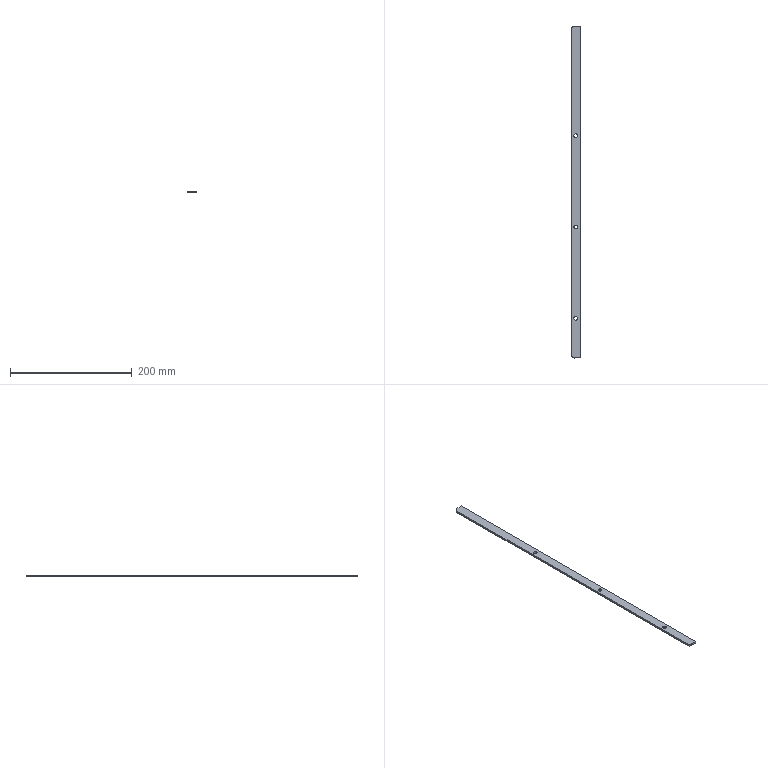Part | STEP file | Input 84 | 1 solid | 14 faces | box 15 x 545 x 3.2 mm | volume 25854 mm3 | cylinder 8 | plane 6 | commonest cylinder face diameters 6 x6 10 x2
STEP:
#1=CARTESIAN_POINT('',(0.,0.,0.));
#2=DIRECTION('',(0.,0.,1.));
#3=DIRECTION('',(1.,0.,0.));
#4=AXIS2_PLACEMENT_3D('',#1,#2,#3);
#5=CARTESIAN_POINT('',(4178.948,425.,2.794));
#6=VERTEX_POINT('',#5);
#7=CARTESIAN_POINT('',(4178.948,425.,-0.4063));
#8=VERTEX_POINT('',#7);
#9=CARTESIAN_POINT('',(4178.948,425.,2.795));
#10=DIRECTION('',(0.,0.,-1.));
#11=VECTOR('',#10,1.);
#12=LINE('',#9,#11);
#13=CARTESIAN_POINT('',(4175.948,425.,2.795));
#14=DIRECTION('',(0.,0.,-1.));
#15=DIRECTION('',(1.,0.,0.));
#16=AXIS2_PLACEMENT_3D('',#13,#14,#15);
#17=CYLINDRICAL_SURFACE('',#16,3.);
#18=CARTESIAN_POINT('',(6.283,0.));
#19=DIRECTION('',(0.,1.));
#20=VECTOR('',#19,1.);
#21=LINE('',#18,#20);
#22=(GEOMETRIC_REPRESENTATION_CONTEXT(2)PARAMETRIC_REPRESENTATION_CONTEXT()REPRESENTATION_CONTEXT('',''));
#23=DEFINITIONAL_REPRESENTATION('',(#21),#22);
#24=PCURVE('',#17,#23);
#25=CARTESIAN_POINT('',(4175.948,425.,2.795));
#26=DIRECTION('',(0.,0.,-1.));
#27=DIRECTION('',(1.,0.,0.));
#28=AXIS2_PLACEMENT_3D('',#25,#26,#27);
#29=CYLINDRICAL_SURFACE('',#28,3.);
#30=CARTESIAN_POINT('',(0.,0.));
#31=DIRECTION('',(0.,1.));
#32=VECTOR('',#31,1.);
#33=LINE('',#30,#32);
#34=(GEOMETRIC_REPRESENTATION_CONTEXT(2)PARAMETRIC_REPRESENTATION_CONTEXT()REPRESENTATION_CONTEXT('',''));
#35=DEFINITIONAL_REPRESENTATION('',(#33),#34);
#36=PCURVE('',#29,#35);
#37=SURFACE_CURVE('',#12,(#24,#36),.PCURVE_S1.);
#38=EDGE_CURVE('',#6,#8,#37,.T.);
#39=ORIENTED_EDGE('',*,*,#38,.T.);
#40=CARTESIAN_POINT('',(4172.948,425.,-0.4063));
#41=VERTEX_POINT('',#40);
#42=CARTESIAN_POINT('',(4175.948,425.,-0.4063));
#43=DIRECTION('',(0.,0.,1.));
#44=DIRECTION('',(1.,0.,0.));
#45=AXIS2_PLACEMENT_3D('',#42,#43,#44);
#46=CIRCLE('',#45,3.);
#47=CARTESIAN_POINT('',(6.283,3.201));
#48=DIRECTION('',(-1.,0.));
#49=VECTOR('',#48,1.);
#50=LINE('',#47,#49);
#51=(GEOMETRIC_REPRESENTATION_CONTEXT(2)PARAMETRIC_REPRESENTATION_CONTEXT()REPRESENTATION_CONTEXT('',''));
#52=DEFINITIONAL_REPRESENTATION('',(#50),#51);
#53=PCURVE('',#17,#52);
#54=CARTESIAN_POINT('',(4173.948,600.,-0.4063));
#55=DIRECTION('',(0.,0.,-1.));
#56=DIRECTION('',(1.,0.,0.));
#57=AXIS2_PLACEMENT_3D('',#54,#55,#56);
#58=PLANE('',#57);
#59=CARTESIAN_POINT('',(5.,175.));
#60=CARTESIAN_POINT('',(5.,169.804));
#61=CARTESIAN_POINT('',(0.5,172.402));
#62=CARTESIAN_POINT('',(-4.,175.));
#63=CARTESIAN_POINT('',(0.5,177.598));
#64=CARTESIAN_POINT('',(5.,180.196));
#65=CARTESIAN_POINT('',(5.,175.));
#66=(BOUNDED_CURVE()B_SPLINE_CURVE(2,(#59,#60,#61,#62,#63,#64,#65),.UNSPECIFIED.,.T.,.F.)B_SPLINE_CURVE_WITH_KNOTS((1,2,2,2,2,1),(-2.094,0.,2.094,4.189,6.283,8.378),.UNSPECIFIED.)CURVE()GEOMETRIC_REPRESENTATION_ITEM()RATIONAL_B_SPLINE_CURVE((1.,0.5,1.,0.5,1.,0.5,1.))REPRESENTATION_ITEM(''));
#67=(GEOMETRIC_REPRESENTATION_CONTEXT(2)PARAMETRIC_REPRESENTATION_CONTEXT()REPRESENTATION_CONTEXT('',''));
#68=DEFINITIONAL_REPRESENTATION('',(#66),#67);
#69=PCURVE('',#58,#68);
#70=SURFACE_CURVE('',#46,(#53,#69),.PCURVE_S1.);
#71=EDGE_CURVE('',#8,#41,#70,.T.);
#72=ORIENTED_EDGE('',*,*,#71,.T.);
#73=CARTESIAN_POINT('',(4172.948,425.,2.794));
#74=VERTEX_POINT('',#73);
#75=CARTESIAN_POINT('',(4172.948,425.,2.795));
#76=DIRECTION('',(0.,0.,-1.));
#77=VECTOR('',#76,1.);
#78=LINE('',#75,#77);
#79=CARTESIAN_POINT('',(3.142,0.));
#80=DIRECTION('',(0.,1.));
#81=VECTOR('',#80,1.);
#82=LINE('',#79,#81);
#83=(GEOMETRIC_REPRESENTATION_CONTEXT(2)PARAMETRIC_REPRESENTATION_CONTEXT()REPRESENTATION_CONTEXT('',''));
#84=DEFINITIONAL_REPRESENTATION('',(#82),#83);
#85=PCURVE('',#17,#84);
#86=CARTESIAN_POINT('',(3.142,0.));
#87=DIRECTION('',(0.,1.));
#88=VECTOR('',#87,1.);
#89=LINE('',#86,#88);
#90=(GEOMETRIC_REPRESENTATION_CONTEXT(2)PARAMETRIC_REPRESENTATION_CONTEXT()REPRESENTATION_CONTEXT('',''));
#91=DEFINITIONAL_REPRESENTATION('',(#89),#90);
#92=PCURVE('',#29,#91);
#93=SURFACE_CURVE('',#78,(#85,#92),.PCURVE_S1.);
#94=EDGE_CURVE('',#74,#41,#93,.T.);
#95=ORIENTED_EDGE('',*,*,#94,.F.);
#96=CARTESIAN_POINT('',(4175.948,425.,2.794));
#97=DIRECTION('',(0.,0.,-1.));
#98=DIRECTION('',(1.,0.,0.));
#99=AXIS2_PLACEMENT_3D('',#96,#97,#98);
#100=CIRCLE('',#99,3.);
#101=CARTESIAN_POINT('',(0.,0.001));
#102=DIRECTION('',(1.,0.));
#103=VECTOR('',#102,1.);
#104=LINE('',#101,#103);
#105=(GEOMETRIC_REPRESENTATION_CONTEXT(2)PARAMETRIC_REPRESENTATION_CONTEXT()REPRESENTATION_CONTEXT('',''));
#106=DEFINITIONAL_REPRESENTATION('',(#104),#105);
#107=PCURVE('',#17,#106);
#108=CARTESIAN_POINT('',(4173.948,600.,2.794));
#109=DIRECTION('',(0.,0.,-1.));
#110=DIRECTION('',(1.,0.,0.));
#111=AXIS2_PLACEMENT_3D('',#108,#109,#110);
#112=PLANE('',#111);
#113=CARTESIAN_POINT('',(2.,175.));
#114=DIRECTION('',(1.,0.));
#115=AXIS2_PLACEMENT_2D('',#113,#114);
#116=CIRCLE('',#115,3.);
#117=(GEOMETRIC_REPRESENTATION_CONTEXT(2)PARAMETRIC_REPRESENTATION_CONTEXT()REPRESENTATION_CONTEXT('',''));
#118=DEFINITIONAL_REPRESENTATION('',(#116),#117);
#119=PCURVE('',#112,#118);
#120=SURFACE_CURVE('',#100,(#107,#119),.PCURVE_S1.);
#121=EDGE_CURVE('',#74,#6,#120,.T.);
#122=ORIENTED_EDGE('',*,*,#121,.T.);
#123=EDGE_LOOP('',(#39,#72,#95,#122));
#124=FACE_BOUND('',#123,.F.);
#125=ADVANCED_FACE('',(#124),#17,.F.);
#126=CARTESIAN_POINT('',(4178.948,125.,2.794));
#127=VERTEX_POINT('',#126);
#128=CARTESIAN_POINT('',(4178.948,125.,-0.4063));
#129=VERTEX_POINT('',#128);
#130=CARTESIAN_POINT('',(4178.948,125.,2.795));
#131=DIRECTION('',(0.,0.,-1.));
#132=VECTOR('',#131,1.);
#133=LINE('',#130,#132);
#134=CARTESIAN_POINT('',(4175.948,125.,2.795));
#135=DIRECTION('',(0.,0.,-1.));
#136=DIRECTION('',(1.,0.,0.));
#137=AXIS2_PLACEMENT_3D('',#134,#135,#136);
#138=CYLINDRICAL_SURFACE('',#137,3.);
#139=CARTESIAN_POINT('',(6.283,0.));
#140=DIRECTION('',(0.,1.));
#141=VECTOR('',#140,1.);
#142=LINE('',#139,#141);
#143=(GEOMETRIC_REPRESENTATION_CONTEXT(2)PARAMETRIC_REPRESENTATION_CONTEXT()REPRESENTATION_CONTEXT('',''));
#144=DEFINITIONAL_REPRESENTATION('',(#142),#143);
#145=PCURVE('',#138,#144);
#146=CARTESIAN_POINT('',(4175.948,125.,2.795));
#147=DIRECTION('',(0.,0.,-1.));
#148=DIRECTION('',(1.,0.,0.));
#149=AXIS2_PLACEMENT_3D('',#146,#147,#148);
#150=CYLINDRICAL_SURFACE('',#149,3.);
#151=CARTESIAN_POINT('',(0.,0.));
#152=DIRECTION('',(0.,1.));
#153=VECTOR('',#152,1.);
#154=LINE('',#151,#153);
#155=(GEOMETRIC_REPRESENTATION_CONTEXT(2)PARAMETRIC_REPRESENTATION_CONTEXT()REPRESENTATION_CONTEXT('',''));
#156=DEFINITIONAL_REPRESENTATION('',(#154),#155);
#157=PCURVE('',#150,#156);
#158=SURFACE_CURVE('',#133,(#145,#157),.PCURVE_S1.);
#159=EDGE_CURVE('',#127,#129,#158,.T.);
#160=ORIENTED_EDGE('',*,*,#159,.T.);
#161=CARTESIAN_POINT('',(4172.948,125.,-0.4063));
#162=VERTEX_POINT('',#161);
#163=CARTESIAN_POINT('',(4175.948,125.,-0.4063));
#164=DIRECTION('',(0.,0.,1.));
#165=DIRECTION('',(1.,0.,0.));
#166=AXIS2_PLACEMENT_3D('',#163,#164,#165);
#167=CIRCLE('',#166,3.);
#168=CARTESIAN_POINT('',(6.283,3.201));
#169=DIRECTION('',(-1.,0.));
#170=VECTOR('',#169,1.);
#171=LINE('',#168,#170);
#172=(GEOMETRIC_REPRESENTATION_CONTEXT(2)PARAMETRIC_REPRESENTATION_CONTEXT()REPRESENTATION_CONTEXT('',''));
#173=DEFINITIONAL_REPRESENTATION('',(#171),#172);
#174=PCURVE('',#138,#173);
#175=CARTESIAN_POINT('',(5.,475.));
#176=CARTESIAN_POINT('',(5.,469.804));
#177=CARTESIAN_POINT('',(0.5,472.402));
#178=CARTESIAN_POINT('',(-4.,475.));
#179=CARTESIAN_POINT('',(0.5,477.598));
#180=CARTESIAN_POINT('',(5.,480.196));
#181=CARTESIAN_POINT('',(5.,475.));
#182=(BOUNDED_CURVE()B_SPLINE_CURVE(2,(#175,#176,#177,#178,#179,#180,#181),.UNSPECIFIED.,.T.,.F.)B_SPLINE_CURVE_WITH_KNOTS((1,2,2,2,2,1),(-2.094,0.,2.094,4.189,6.283,8.378),.UNSPECIFIED.)CURVE()GEOMETRIC_REPRESENTATION_ITEM()RATIONAL_B_SPLINE_CURVE((1.,0.5,1.,0.5,1.,0.5,1.))REPRESENTATION_ITEM(''));
#183=(GEOMETRIC_REPRESENTATION_CONTEXT(2)PARAMETRIC_REPRESENTATION_CONTEXT()REPRESENTATION_CONTEXT('',''));
#184=DEFINITIONAL_REPRESENTATION('',(#182),#183);
#185=PCURVE('',#58,#184);
#186=SURFACE_CURVE('',#167,(#174,#185),.PCURVE_S1.);
#187=EDGE_CURVE('',#129,#162,#186,.T.);
#188=ORIENTED_EDGE('',*,*,#187,.T.);
#189=CARTESIAN_POINT('',(4172.948,125.,2.794));
#190=VERTEX_POINT('',#189);
#191=CARTESIAN_POINT('',(4172.948,125.,2.795));
#192=DIRECTION('',(0.,0.,-1.));
#193=VECTOR('',#192,1.);
#194=LINE('',#191,#193);
#195=CARTESIAN_POINT('',(3.142,0.));
#196=DIRECTION('',(0.,1.));
#197=VECTOR('',#196,1.);
#198=LINE('',#195,#197);
#199=(GEOMETRIC_REPRESENTATION_CONTEXT(2)PARAMETRIC_REPRESENTATION_CONTEXT()REPRESENTATION_CONTEXT('',''));
#200=DEFINITIONAL_REPRESENTATION('',(#198),#199);
#201=PCURVE('',#138,#200);
#202=CARTESIAN_POINT('',(3.142,0.));
#203=DIRECTION('',(0.,1.));
#204=VECTOR('',#203,1.);
#205=LINE('',#202,#204);
#206=(GEOMETRIC_REPRESENTATION_CONTEXT(2)PARAMETRIC_REPRESENTATION_CONTEXT()REPRESENTATION_CONTEXT('',''));
#207=DEFINITIONAL_REPRESENTATION('',(#205),#206);
#208=PCURVE('',#150,#207);
#209=SURFACE_CURVE('',#194,(#201,#208),.PCURVE_S1.);
#210=EDGE_CURVE('',#190,#162,#209,.T.);
#211=ORIENTED_EDGE('',*,*,#210,.F.);
#212=CARTESIAN_POINT('',(4175.948,125.,2.794));
#213=DIRECTION('',(0.,0.,-1.));
#214=DIRECTION('',(1.,0.,0.));
#215=AXIS2_PLACEMENT_3D('',#212,#213,#214);
#216=CIRCLE('',#215,3.);
#217=CARTESIAN_POINT('',(0.,0.001));
#218=DIRECTION('',(1.,0.));
#219=VECTOR('',#218,1.);
#220=LINE('',#217,#219);
#221=(GEOMETRIC_REPRESENTATION_CONTEXT(2)PARAMETRIC_REPRESENTATION_CONTEXT()REPRESENTATION_CONTEXT('',''));
#222=DEFINITIONAL_REPRESENTATION('',(#220),#221);
#223=PCURVE('',#138,#222);
#224=CARTESIAN_POINT('',(2.,475.));
#225=DIRECTION('',(1.,0.));
#226=AXIS2_PLACEMENT_2D('',#224,#225);
#227=CIRCLE('',#226,3.);
#228=(GEOMETRIC_REPRESENTATION_CONTEXT(2)PARAMETRIC_REPRESENTATION_CONTEXT()REPRESENTATION_CONTEXT('',''));
#229=DEFINITIONAL_REPRESENTATION('',(#227),#228);
#230=PCURVE('',#112,#229);
#231=SURFACE_CURVE('',#216,(#223,#230),.PCURVE_S1.);
#232=EDGE_CURVE('',#190,#127,#231,.T.);
#233=ORIENTED_EDGE('',*,*,#232,.T.);
#234=EDGE_LOOP('',(#160,#188,#211,#233));
#235=FACE_BOUND('',#234,.F.);
#236=ADVANCED_FACE('',(#235),#138,.F.);
#237=CARTESIAN_POINT('',(4178.948,275.,2.794));
#238=VERTEX_POINT('',#237);
#239=CARTESIAN_POINT('',(4178.948,275.,-0.4063));
#240=VERTEX_POINT('',#239);
#241=CARTESIAN_POINT('',(4178.948,275.,2.795));
#242=DIRECTION('',(0.,0.,-1.));
#243=VECTOR('',#242,1.);
#244=LINE('',#241,#243);
#245=CARTESIAN_POINT('',(4175.948,275.,2.795));
#246=DIRECTION('',(0.,0.,-1.));
#247=DIRECTION('',(1.,0.,0.));
#248=AXIS2_PLACEMENT_3D('',#245,#246,#247);
#249=CYLINDRICAL_SURFACE('',#248,3.);
#250=CARTESIAN_POINT('',(6.283,0.));
#251=DIRECTION('',(0.,1.));
#252=VECTOR('',#251,1.);
#253=LINE('',#250,#252);
#254=(GEOMETRIC_REPRESENTATION_CONTEXT(2)PARAMETRIC_REPRESENTATION_CONTEXT()REPRESENTATION_CONTEXT('',''));
#255=DEFINITIONAL_REPRESENTATION('',(#253),#254);
#256=PCURVE('',#249,#255);
#257=CARTESIAN_POINT('',(4175.948,275.,2.795));
#258=DIRECTION('',(0.,0.,-1.));
#259=DIRECTION('',(1.,0.,0.));
#260=AXIS2_PLACEMENT_3D('',#257,#258,#259);
#261=CYLINDRICAL_SURFACE('',#260,3.);
#262=CARTESIAN_POINT('',(0.,0.));
#263=DIRECTION('',(0.,1.));
#264=VECTOR('',#263,1.);
#265=LINE('',#262,#264);
#266=(GEOMETRIC_REPRESENTATION_CONTEXT(2)PARAMETRIC_REPRESENTATION_CONTEXT()REPRESENTATION_CONTEXT('',''));
#267=DEFINITIONAL_REPRESENTATION('',(#265),#266);
#268=PCURVE('',#261,#267);
#269=SURFACE_CURVE('',#244,(#256,#268),.PCURVE_S1.);
#270=EDGE_CURVE('',#238,#240,#269,.T.);
#271=ORIENTED_EDGE('',*,*,#270,.T.);
#272=CARTESIAN_POINT('',(4172.948,275.,-0.4063));
#273=VERTEX_POINT('',#272);
#274=CARTESIAN_POINT('',(4175.948,275.,-0.4063));
#275=DIRECTION('',(0.,0.,1.));
#276=DIRECTION('',(1.,0.,0.));
#277=AXIS2_PLACEMENT_3D('',#274,#275,#276);
#278=CIRCLE('',#277,3.);
#279=CARTESIAN_POINT('',(6.283,3.201));
#280=DIRECTION('',(-1.,0.));
#281=VECTOR('',#280,1.);
#282=LINE('',#279,#281);
#283=(GEOMETRIC_REPRESENTATION_CONTEXT(2)PARAMETRIC_REPRESENTATION_CONTEXT()REPRESENTATION_CONTEXT('',''));
#284=DEFINITIONAL_REPRESENTATION('',(#282),#283);
#285=PCURVE('',#249,#284);
#286=CARTESIAN_POINT('',(5.,325.));
#287=CARTESIAN_POINT('',(5.,319.804));
#288=CARTESIAN_POINT('',(0.5,322.402));
#289=CARTESIAN_POINT('',(-4.,325.));
#290=CARTESIAN_POINT('',(0.5,327.598));
#291=CARTESIAN_POINT('',(5.,330.196));
#292=CARTESIAN_POINT('',(5.,325.));
#293=(BOUNDED_CURVE()B_SPLINE_CURVE(2,(#286,#287,#288,#289,#290,#291,#292),.UNSPECIFIED.,.T.,.F.)B_SPLINE_CURVE_WITH_KNOTS((1,2,2,2,2,1),(-2.094,0.,2.094,4.189,6.283,8.378),.UNSPECIFIED.)CURVE()GEOMETRIC_REPRESENTATION_ITEM()RATIONAL_B_SPLINE_CURVE((1.,0.5,1.,0.5,1.,0.5,1.))REPRESENTATION_ITEM(''));
#294=(GEOMETRIC_REPRESENTATION_CONTEXT(2)PARAMETRIC_REPRESENTATION_CONTEXT()REPRESENTATION_CONTEXT('',''));
#295=DEFINITIONAL_REPRESENTATION('',(#293),#294);
#296=PCURVE('',#58,#295);
#297=SURFACE_CURVE('',#278,(#285,#296),.PCURVE_S1.);
#298=EDGE_CURVE('',#240,#273,#297,.T.);
#299=ORIENTED_EDGE('',*,*,#298,.T.);
#300=CARTESIAN_POINT('',(4172.948,275.,2.794));
#301=VERTEX_POINT('',#300);
#302=CARTESIAN_POINT('',(4172.948,275.,2.795));
#303=DIRECTION('',(0.,0.,-1.));
#304=VECTOR('',#303,1.);
#305=LINE('',#302,#304);
#306=CARTESIAN_POINT('',(3.142,0.));
#307=DIRECTION('',(0.,1.));
#308=VECTOR('',#307,1.);
#309=LINE('',#306,#308);
#310=(GEOMETRIC_REPRESENTATION_CONTEXT(2)PARAMETRIC_REPRESENTATION_CONTEXT()REPRESENTATION_CONTEXT('',''));
#311=DEFINITIONAL_REPRESENTATION('',(#309),#310);
#312=PCURVE('',#249,#311);
#313=CARTESIAN_POINT('',(3.142,0.));
#314=DIRECTION('',(0.,1.));
#315=VECTOR('',#314,1.);
#316=LINE('',#313,#315);
#317=(GEOMETRIC_REPRESENTATION_CONTEXT(2)PARAMETRIC_REPRESENTATION_CONTEXT()REPRESENTATION_CONTEXT('',''));
#318=DEFINITIONAL_REPRESENTATION('',(#316),#317);
#319=PCURVE('',#261,#318);
#320=SURFACE_CURVE('',#305,(#312,#319),.PCURVE_S1.);
#321=EDGE_CURVE('',#301,#273,#320,.T.);
#322=ORIENTED_EDGE('',*,*,#321,.F.);
#323=CARTESIAN_POINT('',(4175.948,275.,2.794));
#324=DIRECTION('',(0.,0.,-1.));
#325=DIRECTION('',(1.,0.,0.));
#326=AXIS2_PLACEMENT_3D('',#323,#324,#325);
#327=CIRCLE('',#326,3.);
#328=CARTESIAN_POINT('',(0.,0.001));
#329=DIRECTION('',(1.,0.));
#330=VECTOR('',#329,1.);
#331=LINE('',#328,#330);
#332=(GEOMETRIC_REPRESENTATION_CONTEXT(2)PARAMETRIC_REPRESENTATION_CONTEXT()REPRESENTATION_CONTEXT('',''));
#333=DEFINITIONAL_REPRESENTATION('',(#331),#332);
#334=PCURVE('',#249,#333);
#335=CARTESIAN_POINT('',(2.,325.));
#336=DIRECTION('',(1.,0.));
#337=AXIS2_PLACEMENT_2D('',#335,#336);
#338=CIRCLE('',#337,3.);
#339=(GEOMETRIC_REPRESENTATION_CONTEXT(2)PARAMETRIC_REPRESENTATION_CONTEXT()REPRESENTATION_CONTEXT('',''));
#340=DEFINITIONAL_REPRESENTATION('',(#338),#339);
#341=PCURVE('',#112,#340);
#342=SURFACE_CURVE('',#327,(#334,#341),.PCURVE_S1.);
#343=EDGE_CURVE('',#301,#238,#342,.T.);
#344=ORIENTED_EDGE('',*,*,#343,.T.);
#345=EDGE_LOOP('',(#271,#299,#322,#344));
#346=FACE_BOUND('',#345,.F.);
#347=ADVANCED_FACE('',(#346),#249,.F.);
#348=CARTESIAN_POINT('',(4183.948,605.,-0.4063));
#349=VERTEX_POINT('',#348);
#350=CARTESIAN_POINT('',(4173.948,605.,-0.4063));
#351=VERTEX_POINT('',#350);
#352=CARTESIAN_POINT('',(4183.948,605.,-0.4063));
#353=DIRECTION('',(-1.,0.,0.));
#354=VECTOR('',#353,1.);
#355=LINE('',#352,#354);
#356=CARTESIAN_POINT('',(4183.948,605.,2.794));
#357=DIRECTION('',(0.,1.,0.));
#358=DIRECTION('',(-1.,0.,0.));
#359=AXIS2_PLACEMENT_3D('',#356,#357,#358);
#360=PLANE('',#359);
#361=CARTESIAN_POINT('',(0.,-3.2));
#362=DIRECTION('',(1.,0.));
#363=VECTOR('',#362,1.);
#364=LINE('',#361,#363);
#365=(GEOMETRIC_REPRESENTATION_CONTEXT(2)PARAMETRIC_REPRESENTATION_CONTEXT()REPRESENTATION_CONTEXT('',''));
#366=DEFINITIONAL_REPRESENTATION('',(#364),#365);
#367=PCURVE('',#360,#366);
#368=CARTESIAN_POINT('',(10.,-5.));
#369=DIRECTION('',(-1.,0.));
#370=VECTOR('',#369,1.);
#371=LINE('',#368,#370);
#372=(GEOMETRIC_REPRESENTATION_CONTEXT(2)PARAMETRIC_REPRESENTATION_CONTEXT()REPRESENTATION_CONTEXT('',''));
#373=DEFINITIONAL_REPRESENTATION('',(#371),#372);
#374=PCURVE('',#58,#373);
#375=SURFACE_CURVE('',#355,(#367,#374),.PCURVE_S1.);
#376=EDGE_CURVE('',#349,#351,#375,.T.);
#377=ORIENTED_EDGE('',*,*,#376,.T.);
#378=CARTESIAN_POINT('',(4173.948,605.,2.794));
#379=VERTEX_POINT('',#378);
#380=CARTESIAN_POINT('',(4173.948,605.,2.794));
#381=DIRECTION('',(0.,0.,-1.));
#382=VECTOR('',#381,1.);
#383=LINE('',#380,#382);
#384=CARTESIAN_POINT('',(10.,0.));
#385=DIRECTION('',(0.,-1.));
#386=VECTOR('',#385,1.);
#387=LINE('',#384,#386);
#388=(GEOMETRIC_REPRESENTATION_CONTEXT(2)PARAMETRIC_REPRESENTATION_CONTEXT()REPRESENTATION_CONTEXT('',''));
#389=DEFINITIONAL_REPRESENTATION('',(#387),#388);
#390=PCURVE('',#360,#389);
#391=CARTESIAN_POINT('',(4173.948,600.,2.794));
#392=DIRECTION('',(0.,0.,-1.));
#393=DIRECTION('',(1.,0.,0.));
#394=AXIS2_PLACEMENT_3D('',#391,#392,#393);
#395=CYLINDRICAL_SURFACE('',#394,5.);
#396=CARTESIAN_POINT('',(4.712,0.));
#397=DIRECTION('',(0.,1.));
#398=VECTOR('',#397,1.);
#399=LINE('',#396,#398);
#400=(GEOMETRIC_REPRESENTATION_CONTEXT(2)PARAMETRIC_REPRESENTATION_CONTEXT()REPRESENTATION_CONTEXT('',''));
#401=DEFINITIONAL_REPRESENTATION('',(#399),#400);
#402=PCURVE('',#395,#401);
#403=SURFACE_CURVE('',#383,(#390,#402),.PCURVE_S1.);
#404=EDGE_CURVE('',#379,#351,#403,.T.);
#405=ORIENTED_EDGE('',*,*,#404,.F.);
#406=CARTESIAN_POINT('',(4183.948,605.,2.794));
#407=VERTEX_POINT('',#406);
#408=CARTESIAN_POINT('',(4183.948,605.,2.794));
#409=DIRECTION('',(-1.,0.,0.));
#410=VECTOR('',#409,1.);
#411=LINE('',#408,#410);
#412=CARTESIAN_POINT('',(0.,0.));
#413=DIRECTION('',(1.,0.));
#414=VECTOR('',#413,1.);
#415=LINE('',#412,#414);
#416=(GEOMETRIC_REPRESENTATION_CONTEXT(2)PARAMETRIC_REPRESENTATION_CONTEXT()REPRESENTATION_CONTEXT('',''));
#417=DEFINITIONAL_REPRESENTATION('',(#415),#416);
#418=PCURVE('',#360,#417);
#419=CARTESIAN_POINT('',(10.,-5.));
#420=DIRECTION('',(-1.,0.));
#421=VECTOR('',#420,1.);
#422=LINE('',#419,#421);
#423=(GEOMETRIC_REPRESENTATION_CONTEXT(2)PARAMETRIC_REPRESENTATION_CONTEXT()REPRESENTATION_CONTEXT('',''));
#424=DEFINITIONAL_REPRESENTATION('',(#422),#423);
#425=PCURVE('',#112,#424);
#426=SURFACE_CURVE('',#411,(#418,#425),.PCURVE_S1.);
#427=EDGE_CURVE('',#407,#379,#426,.T.);
#428=ORIENTED_EDGE('',*,*,#427,.F.);
#429=CARTESIAN_POINT('',(4183.948,605.,2.794));
#430=DIRECTION('',(0.,0.,-1.));
#431=VECTOR('',#430,1.);
#432=LINE('',#429,#431);
#433=CARTESIAN_POINT('',(0.,0.));
#434=DIRECTION('',(0.,-1.));
#435=VECTOR('',#434,1.);
#436=LINE('',#433,#435);
#437=(GEOMETRIC_REPRESENTATION_CONTEXT(2)PARAMETRIC_REPRESENTATION_CONTEXT()REPRESENTATION_CONTEXT('',''));
#438=DEFINITIONAL_REPRESENTATION('',(#436),#437);
#439=PCURVE('',#360,#438);
#440=CARTESIAN_POINT('',(4183.948,605.,2.794));
#441=DIRECTION('',(1.,0.,0.));
#442=DIRECTION('',(0.,1.,0.));
#443=AXIS2_PLACEMENT_3D('',#440,#441,#442);
#444=PLANE('',#443);
#445=CARTESIAN_POINT('',(0.,0.));
#446=DIRECTION('',(0.,-1.));
#447=VECTOR('',#446,1.);
#448=LINE('',#445,#447);
#449=(GEOMETRIC_REPRESENTATION_CONTEXT(2)PARAMETRIC_REPRESENTATION_CONTEXT()REPRESENTATION_CONTEXT('',''));
#450=DEFINITIONAL_REPRESENTATION('',(#448),#449);
#451=PCURVE('',#444,#450);
#452=SURFACE_CURVE('',#432,(#439,#451),.PCURVE_S1.);
#453=EDGE_CURVE('',#407,#349,#452,.T.);
#454=ORIENTED_EDGE('',*,*,#453,.T.);
#455=EDGE_LOOP('',(#377,#405,#428,#454));
#456=FACE_BOUND('',#455,.T.);
#457=ADVANCED_FACE('',(#456),#360,.T.);
#458=CARTESIAN_POINT('',(4183.948,60.,-0.4063));
#459=VERTEX_POINT('',#458);
#460=CARTESIAN_POINT('',(4183.948,605.,-0.4063));
#461=DIRECTION('',(0.,1.,0.));
#462=VECTOR('',#461,1.);
#463=LINE('',#460,#462);
#464=CARTESIAN_POINT('',(0.,-3.2));
#465=DIRECTION('',(1.,0.));
#466=VECTOR('',#465,1.);
#467=LINE('',#464,#466);
#468=(GEOMETRIC_REPRESENTATION_CONTEXT(2)PARAMETRIC_REPRESENTATION_CONTEXT()REPRESENTATION_CONTEXT('',''));
#469=DEFINITIONAL_REPRESENTATION('',(#467),#468);
#470=PCURVE('',#444,#469);
#471=CARTESIAN_POINT('',(10.,-5.));
#472=DIRECTION('',(0.,-1.));
#473=VECTOR('',#472,1.);
#474=LINE('',#471,#473);
#475=(GEOMETRIC_REPRESENTATION_CONTEXT(2)PARAMETRIC_REPRESENTATION_CONTEXT()REPRESENTATION_CONTEXT('',''));
#476=DEFINITIONAL_REPRESENTATION('',(#474),#475);
#477=PCURVE('',#58,#476);
#478=SURFACE_CURVE('',#463,(#470,#477),.PCURVE_S1.);
#479=EDGE_CURVE('',#459,#349,#478,.T.);
#480=ORIENTED_EDGE('',*,*,#479,.T.);
#481=ORIENTED_EDGE('',*,*,#453,.F.);
#482=CARTESIAN_POINT('',(4183.948,60.,2.794));
#483=VERTEX_POINT('',#482);
#484=CARTESIAN_POINT('',(4183.948,605.,2.794));
#485=DIRECTION('',(0.,1.,0.));
#486=VECTOR('',#485,1.);
#487=LINE('',#484,#486);
#488=CARTESIAN_POINT('',(0.,0.));
#489=DIRECTION('',(1.,0.));
#490=VECTOR('',#489,1.);
#491=LINE('',#488,#490);
#492=(GEOMETRIC_REPRESENTATION_CONTEXT(2)PARAMETRIC_REPRESENTATION_CONTEXT()REPRESENTATION_CONTEXT('',''));
#493=DEFINITIONAL_REPRESENTATION('',(#491),#492);
#494=PCURVE('',#444,#493);
#495=CARTESIAN_POINT('',(10.,-5.));
#496=DIRECTION('',(0.,-1.));
#497=VECTOR('',#496,1.);
#498=LINE('',#495,#497);
#499=(GEOMETRIC_REPRESENTATION_CONTEXT(2)PARAMETRIC_REPRESENTATION_CONTEXT()REPRESENTATION_CONTEXT('',''));
#500=DEFINITIONAL_REPRESENTATION('',(#498),#499);
#501=PCURVE('',#112,#500);
#502=SURFACE_CURVE('',#487,(#494,#501),.PCURVE_S1.);
#503=EDGE_CURVE('',#483,#407,#502,.T.);
#504=ORIENTED_EDGE('',*,*,#503,.F.);
#505=CARTESIAN_POINT('',(4183.948,60.,2.794));
#506=DIRECTION('',(0.,0.,-1.));
#507=VECTOR('',#506,1.);
#508=LINE('',#505,#507);
#509=CARTESIAN_POINT('',(-545.,0.));
#510=DIRECTION('',(0.,-1.));
#511=VECTOR('',#510,1.);
#512=LINE('',#509,#511);
#513=(GEOMETRIC_REPRESENTATION_CONTEXT(2)PARAMETRIC_REPRESENTATION_CONTEXT()REPRESENTATION_CONTEXT('',''));
#514=DEFINITIONAL_REPRESENTATION('',(#512),#513);
#515=PCURVE('',#444,#514);
#516=CARTESIAN_POINT('',(4183.948,60.,2.794));
#517=DIRECTION('',(0.,-1.,0.));
#518=DIRECTION('',(1.,0.,0.));
#519=AXIS2_PLACEMENT_3D('',#516,#517,#518);
#520=PLANE('',#519);
#521=CARTESIAN_POINT('',(0.,0.));
#522=DIRECTION('',(0.,-1.));
#523=VECTOR('',#522,1.);
#524=LINE('',#521,#523);
#525=(GEOMETRIC_REPRESENTATION_CONTEXT(2)PARAMETRIC_REPRESENTATION_CONTEXT()REPRESENTATION_CONTEXT('',''));
#526=DEFINITIONAL_REPRESENTATION('',(#524),#525);
#527=PCURVE('',#520,#526);
#528=SURFACE_CURVE('',#508,(#515,#527),.PCURVE_S1.);
#529=EDGE_CURVE('',#483,#459,#528,.T.);
#530=ORIENTED_EDGE('',*,*,#529,.T.);
#531=EDGE_LOOP('',(#480,#481,#504,#530));
#532=FACE_BOUND('',#531,.T.);
#533=ADVANCED_FACE('',(#532),#444,.T.);
#534=CARTESIAN_POINT('',(4173.948,60.,-0.4063));
#535=VERTEX_POINT('',#534);
#536=CARTESIAN_POINT('',(4183.948,60.,-0.4063));
#537=DIRECTION('',(1.,0.,0.));
#538=VECTOR('',#537,1.);
#539=LINE('',#536,#538);
#540=CARTESIAN_POINT('',(0.,-3.2));
#541=DIRECTION('',(1.,0.));
#542=VECTOR('',#541,1.);
#543=LINE('',#540,#542);
#544=(GEOMETRIC_REPRESENTATION_CONTEXT(2)PARAMETRIC_REPRESENTATION_CONTEXT()REPRESENTATION_CONTEXT('',''));
#545=DEFINITIONAL_REPRESENTATION('',(#543),#544);
#546=PCURVE('',#520,#545);
#547=CARTESIAN_POINT('',(10.,540.));
#548=DIRECTION('',(1.,0.));
#549=VECTOR('',#548,1.);
#550=LINE('',#547,#549);
#551=(GEOMETRIC_REPRESENTATION_CONTEXT(2)PARAMETRIC_REPRESENTATION_CONTEXT()REPRESENTATION_CONTEXT('',''));
#552=DEFINITIONAL_REPRESENTATION('',(#550),#551);
#553=PCURVE('',#58,#552);
#554=SURFACE_CURVE('',#539,(#546,#553),.PCURVE_S1.);
#555=EDGE_CURVE('',#535,#459,#554,.T.);
#556=ORIENTED_EDGE('',*,*,#555,.T.);
#557=ORIENTED_EDGE('',*,*,#529,.F.);
#558=CARTESIAN_POINT('',(4173.948,60.,2.794));
#559=VERTEX_POINT('',#558);
#560=CARTESIAN_POINT('',(4183.948,60.,2.794));
#561=DIRECTION('',(1.,0.,0.));
#562=VECTOR('',#561,1.);
#563=LINE('',#560,#562);
#564=CARTESIAN_POINT('',(0.,0.));
#565=DIRECTION('',(1.,0.));
#566=VECTOR('',#565,1.);
#567=LINE('',#564,#566);
#568=(GEOMETRIC_REPRESENTATION_CONTEXT(2)PARAMETRIC_REPRESENTATION_CONTEXT()REPRESENTATION_CONTEXT('',''));
#569=DEFINITIONAL_REPRESENTATION('',(#567),#568);
#570=PCURVE('',#520,#569);
#571=CARTESIAN_POINT('',(10.,540.));
#572=DIRECTION('',(1.,0.));
#573=VECTOR('',#572,1.);
#574=LINE('',#571,#573);
#575=(GEOMETRIC_REPRESENTATION_CONTEXT(2)PARAMETRIC_REPRESENTATION_CONTEXT()REPRESENTATION_CONTEXT('',''));
#576=DEFINITIONAL_REPRESENTATION('',(#574),#575);
#577=PCURVE('',#112,#576);
#578=SURFACE_CURVE('',#563,(#570,#577),.PCURVE_S1.);
#579=EDGE_CURVE('',#559,#483,#578,.T.);
#580=ORIENTED_EDGE('',*,*,#579,.F.);
#581=CARTESIAN_POINT('',(4173.948,60.,2.794));
#582=DIRECTION('',(0.,0.,-1.));
#583=VECTOR('',#582,1.);
#584=LINE('',#581,#583);
#585=CARTESIAN_POINT('',(-10.,0.));
#586=DIRECTION('',(0.,-1.));
#587=VECTOR('',#586,1.);
#588=LINE('',#585,#587);
#589=(GEOMETRIC_REPRESENTATION_CONTEXT(2)PARAMETRIC_REPRESENTATION_CONTEXT()REPRESENTATION_CONTEXT('',''));
#590=DEFINITIONAL_REPRESENTATION('',(#588),#589);
#591=PCURVE('',#520,#590);
#592=CARTESIAN_POINT('',(4173.948,65.,2.794));
#593=DIRECTION('',(0.,0.,-1.));
#594=DIRECTION('',(1.,0.,0.));
#595=AXIS2_PLACEMENT_3D('',#592,#593,#594);
#596=CYLINDRICAL_SURFACE('',#595,5.);
#597=CARTESIAN_POINT('',(1.571,0.));
#598=DIRECTION('',(0.,1.));
#599=VECTOR('',#598,1.);
#600=LINE('',#597,#599);
#601=(GEOMETRIC_REPRESENTATION_CONTEXT(2)PARAMETRIC_REPRESENTATION_CONTEXT()REPRESENTATION_CONTEXT('',''));
#602=DEFINITIONAL_REPRESENTATION('',(#600),#601);
#603=PCURVE('',#596,#602);
#604=SURFACE_CURVE('',#584,(#591,#603),.PCURVE_S1.);
#605=EDGE_CURVE('',#559,#535,#604,.T.);
#606=ORIENTED_EDGE('',*,*,#605,.T.);
#607=EDGE_LOOP('',(#556,#557,#580,#606));
#608=FACE_BOUND('',#607,.T.);
#609=ADVANCED_FACE('',(#608),#520,.T.);
#610=CARTESIAN_POINT('',(4168.948,65.,-0.4063));
#611=VERTEX_POINT('',#610);
#612=CARTESIAN_POINT('',(4173.948,65.,-0.4063));
#613=DIRECTION('',(0.,0.,1.));
#614=DIRECTION('',(1.,0.,0.));
#615=AXIS2_PLACEMENT_3D('',#612,#613,#614);
#616=CIRCLE('',#615,5.);
#617=CARTESIAN_POINT('',(6.283,3.2));
#618=DIRECTION('',(-1.,0.));
#619=VECTOR('',#618,1.);
#620=LINE('',#617,#619);
#621=(GEOMETRIC_REPRESENTATION_CONTEXT(2)PARAMETRIC_REPRESENTATION_CONTEXT()REPRESENTATION_CONTEXT('',''));
#622=DEFINITIONAL_REPRESENTATION('',(#620),#621);
#623=PCURVE('',#596,#622);
#624=CARTESIAN_POINT('',(5.,535.));
#625=CARTESIAN_POINT('',(5.,526.34));
#626=CARTESIAN_POINT('',(-2.5,530.67));
#627=CARTESIAN_POINT('',(-10.,535.));
#628=CARTESIAN_POINT('',(-2.5,539.33));
#629=CARTESIAN_POINT('',(5.,543.66));
#630=CARTESIAN_POINT('',(5.,535.));
#631=(BOUNDED_CURVE()B_SPLINE_CURVE(2,(#624,#625,#626,#627,#628,#629,#630),.UNSPECIFIED.,.T.,.F.)B_SPLINE_CURVE_WITH_KNOTS((1,2,2,2,2,1),(-2.094,0.,2.094,4.189,6.283,8.378),.UNSPECIFIED.)CURVE()GEOMETRIC_REPRESENTATION_ITEM()RATIONAL_B_SPLINE_CURVE((1.,0.5,1.,0.5,1.,0.5,1.))REPRESENTATION_ITEM(''));
#632=(GEOMETRIC_REPRESENTATION_CONTEXT(2)PARAMETRIC_REPRESENTATION_CONTEXT()REPRESENTATION_CONTEXT('',''));
#633=DEFINITIONAL_REPRESENTATION('',(#631),#632);
#634=PCURVE('',#58,#633);
#635=SURFACE_CURVE('',#616,(#623,#634),.PCURVE_S1.);
#636=EDGE_CURVE('',#611,#535,#635,.T.);
#637=ORIENTED_EDGE('',*,*,#636,.T.);
#638=ORIENTED_EDGE('',*,*,#605,.F.);
#639=CARTESIAN_POINT('',(4168.948,65.,2.794));
#640=VERTEX_POINT('',#639);
#641=CARTESIAN_POINT('',(4173.948,65.,2.794));
#642=DIRECTION('',(0.,0.,1.));
#643=DIRECTION('',(1.,0.,0.));
#644=AXIS2_PLACEMENT_3D('',#641,#642,#643);
#645=CIRCLE('',#644,5.);
#646=CARTESIAN_POINT('',(6.283,0.));
#647=DIRECTION('',(-1.,0.));
#648=VECTOR('',#647,1.);
#649=LINE('',#646,#648);
#650=(GEOMETRIC_REPRESENTATION_CONTEXT(2)PARAMETRIC_REPRESENTATION_CONTEXT()REPRESENTATION_CONTEXT('',''));
#651=DEFINITIONAL_REPRESENTATION('',(#649),#650);
#652=PCURVE('',#596,#651);
#653=CARTESIAN_POINT('',(5.,535.));
#654=CARTESIAN_POINT('',(5.,526.34));
#655=CARTESIAN_POINT('',(-2.5,530.67));
#656=CARTESIAN_POINT('',(-10.,535.));
#657=CARTESIAN_POINT('',(-2.5,539.33));
#658=CARTESIAN_POINT('',(5.,543.66));
#659=CARTESIAN_POINT('',(5.,535.));
#660=(BOUNDED_CURVE()B_SPLINE_CURVE(2,(#653,#654,#655,#656,#657,#658,#659),.UNSPECIFIED.,.T.,.F.)B_SPLINE_CURVE_WITH_KNOTS((1,2,2,2,2,1),(-2.094,0.,2.094,4.189,6.283,8.378),.UNSPECIFIED.)CURVE()GEOMETRIC_REPRESENTATION_ITEM()RATIONAL_B_SPLINE_CURVE((1.,0.5,1.,0.5,1.,0.5,1.))REPRESENTATION_ITEM(''));
#661=(GEOMETRIC_REPRESENTATION_CONTEXT(2)PARAMETRIC_REPRESENTATION_CONTEXT()REPRESENTATION_CONTEXT('',''));
#662=DEFINITIONAL_REPRESENTATION('',(#660),#661);
#663=PCURVE('',#112,#662);
#664=SURFACE_CURVE('',#645,(#652,#663),.PCURVE_S1.);
#665=EDGE_CURVE('',#640,#559,#664,.T.);
#666=ORIENTED_EDGE('',*,*,#665,.F.);
#667=CARTESIAN_POINT('',(4168.948,65.,2.794));
#668=DIRECTION('',(0.,0.,-1.));
#669=VECTOR('',#668,1.);
#670=LINE('',#667,#669);
#671=CARTESIAN_POINT('',(3.142,0.));
#672=DIRECTION('',(0.,1.));
#673=VECTOR('',#672,1.);
#674=LINE('',#671,#673);
#675=(GEOMETRIC_REPRESENTATION_CONTEXT(2)PARAMETRIC_REPRESENTATION_CONTEXT()REPRESENTATION_CONTEXT('',''));
#676=DEFINITIONAL_REPRESENTATION('',(#674),#675);
#677=PCURVE('',#596,#676);
#678=CARTESIAN_POINT('',(4168.948,600.,2.794));
#679=DIRECTION('',(-1.,0.,0.));
#680=DIRECTION('',(0.,-1.,0.));
#681=AXIS2_PLACEMENT_3D('',#678,#679,#680);
#682=PLANE('',#681);
#683=CARTESIAN_POINT('',(535.,0.));
#684=DIRECTION('',(0.,-1.));
#685=VECTOR('',#684,1.);
#686=LINE('',#683,#685);
#687=(GEOMETRIC_REPRESENTATION_CONTEXT(2)PARAMETRIC_REPRESENTATION_CONTEXT()REPRESENTATION_CONTEXT('',''));
#688=DEFINITIONAL_REPRESENTATION('',(#686),#687);
#689=PCURVE('',#682,#688);
#690=SURFACE_CURVE('',#670,(#677,#689),.PCURVE_S1.);
#691=EDGE_CURVE('',#640,#611,#690,.T.);
#692=ORIENTED_EDGE('',*,*,#691,.T.);
#693=EDGE_LOOP('',(#637,#638,#666,#692));
#694=FACE_BOUND('',#693,.T.);
#695=ADVANCED_FACE('',(#694),#596,.T.);
#696=CARTESIAN_POINT('',(4168.948,600.,-0.4063));
#697=VERTEX_POINT('',#696);
#698=CARTESIAN_POINT('',(4168.948,600.,-0.4063));
#699=DIRECTION('',(0.,-1.,0.));
#700=VECTOR('',#699,1.);
#701=LINE('',#698,#700);
#702=CARTESIAN_POINT('',(0.,-3.2));
#703=DIRECTION('',(1.,0.));
#704=VECTOR('',#703,1.);
#705=LINE('',#702,#704);
#706=(GEOMETRIC_REPRESENTATION_CONTEXT(2)PARAMETRIC_REPRESENTATION_CONTEXT()REPRESENTATION_CONTEXT('',''));
#707=DEFINITIONAL_REPRESENTATION('',(#705),#706);
#708=PCURVE('',#682,#707);
#709=CARTESIAN_POINT('',(-5.,0.));
#710=DIRECTION('',(0.,1.));
#711=VECTOR('',#710,1.);
#712=LINE('',#709,#711);
#713=(GEOMETRIC_REPRESENTATION_CONTEXT(2)PARAMETRIC_REPRESENTATION_CONTEXT()REPRESENTATION_CONTEXT('',''));
#714=DEFINITIONAL_REPRESENTATION('',(#712),#713);
#715=PCURVE('',#58,#714);
#716=SURFACE_CURVE('',#701,(#708,#715),.PCURVE_S1.);
#717=EDGE_CURVE('',#697,#611,#716,.T.);
#718=ORIENTED_EDGE('',*,*,#717,.T.);
#719=ORIENTED_EDGE('',*,*,#691,.F.);
#720=CARTESIAN_POINT('',(4168.948,600.,2.794));
#721=VERTEX_POINT('',#720);
#722=CARTESIAN_POINT('',(4168.948,600.,2.794));
#723=DIRECTION('',(0.,-1.,0.));
#724=VECTOR('',#723,1.);
#725=LINE('',#722,#724);
#726=CARTESIAN_POINT('',(0.,0.));
#727=DIRECTION('',(1.,0.));
#728=VECTOR('',#727,1.);
#729=LINE('',#726,#728);
#730=(GEOMETRIC_REPRESENTATION_CONTEXT(2)PARAMETRIC_REPRESENTATION_CONTEXT()REPRESENTATION_CONTEXT('',''));
#731=DEFINITIONAL_REPRESENTATION('',(#729),#730);
#732=PCURVE('',#682,#731);
#733=CARTESIAN_POINT('',(-5.,0.));
#734=DIRECTION('',(0.,1.));
#735=VECTOR('',#734,1.);
#736=LINE('',#733,#735);
#737=(GEOMETRIC_REPRESENTATION_CONTEXT(2)PARAMETRIC_REPRESENTATION_CONTEXT()REPRESENTATION_CONTEXT('',''));
#738=DEFINITIONAL_REPRESENTATION('',(#736),#737);
#739=PCURVE('',#112,#738);
#740=SURFACE_CURVE('',#725,(#732,#739),.PCURVE_S1.);
#741=EDGE_CURVE('',#721,#640,#740,.T.);
#742=ORIENTED_EDGE('',*,*,#741,.F.);
#743=CARTESIAN_POINT('',(4168.948,600.,2.794));
#744=DIRECTION('',(0.,0.,-1.));
#745=VECTOR('',#744,1.);
#746=LINE('',#743,#745);
#747=CARTESIAN_POINT('',(0.,0.));
#748=DIRECTION('',(0.,-1.));
#749=VECTOR('',#748,1.);
#750=LINE('',#747,#749);
#751=(GEOMETRIC_REPRESENTATION_CONTEXT(2)PARAMETRIC_REPRESENTATION_CONTEXT()REPRESENTATION_CONTEXT('',''));
#752=DEFINITIONAL_REPRESENTATION('',(#750),#751);
#753=PCURVE('',#682,#752);
#754=CARTESIAN_POINT('',(3.142,0.));
#755=DIRECTION('',(0.,1.));
#756=VECTOR('',#755,1.);
#757=LINE('',#754,#756);
#758=(GEOMETRIC_REPRESENTATION_CONTEXT(2)PARAMETRIC_REPRESENTATION_CONTEXT()REPRESENTATION_CONTEXT('',''));
#759=DEFINITIONAL_REPRESENTATION('',(#757),#758);
#760=PCURVE('',#395,#759);
#761=SURFACE_CURVE('',#746,(#753,#760),.PCURVE_S1.);
#762=EDGE_CURVE('',#721,#697,#761,.T.);
#763=ORIENTED_EDGE('',*,*,#762,.T.);
#764=EDGE_LOOP('',(#718,#719,#742,#763));
#765=FACE_BOUND('',#764,.T.);
#766=ADVANCED_FACE('',(#765),#682,.T.);
#767=CARTESIAN_POINT('',(4173.948,600.,-0.4063));
#768=DIRECTION('',(0.,0.,1.));
#769=DIRECTION('',(1.,0.,0.));
#770=AXIS2_PLACEMENT_3D('',#767,#768,#769);
#771=CIRCLE('',#770,5.);
#772=CARTESIAN_POINT('',(6.283,3.2));
#773=DIRECTION('',(-1.,0.));
#774=VECTOR('',#773,1.);
#775=LINE('',#772,#774);
#776=(GEOMETRIC_REPRESENTATION_CONTEXT(2)PARAMETRIC_REPRESENTATION_CONTEXT()REPRESENTATION_CONTEXT('',''));
#777=DEFINITIONAL_REPRESENTATION('',(#775),#776);
#778=PCURVE('',#395,#777);
#779=CARTESIAN_POINT('',(5.,0.));
#780=CARTESIAN_POINT('',(5.,-8.66));
#781=CARTESIAN_POINT('',(-2.5,-4.33));
#782=CARTESIAN_POINT('',(-10.,0.));
#783=CARTESIAN_POINT('',(-2.5,4.33));
#784=CARTESIAN_POINT('',(5.,8.66));
#785=CARTESIAN_POINT('',(5.,0.));
#786=(BOUNDED_CURVE()B_SPLINE_CURVE(2,(#779,#780,#781,#782,#783,#784,#785),.UNSPECIFIED.,.T.,.F.)B_SPLINE_CURVE_WITH_KNOTS((1,2,2,2,2,1),(-2.094,0.,2.094,4.189,6.283,8.378),.UNSPECIFIED.)CURVE()GEOMETRIC_REPRESENTATION_ITEM()RATIONAL_B_SPLINE_CURVE((1.,0.5,1.,0.5,1.,0.5,1.))REPRESENTATION_ITEM(''));
#787=(GEOMETRIC_REPRESENTATION_CONTEXT(2)PARAMETRIC_REPRESENTATION_CONTEXT()REPRESENTATION_CONTEXT('',''));
#788=DEFINITIONAL_REPRESENTATION('',(#786),#787);
#789=PCURVE('',#58,#788);
#790=SURFACE_CURVE('',#771,(#778,#789),.PCURVE_S1.);
#791=EDGE_CURVE('',#351,#697,#790,.T.);
#792=ORIENTED_EDGE('',*,*,#791,.T.);
#793=ORIENTED_EDGE('',*,*,#762,.F.);
#794=CARTESIAN_POINT('',(4173.948,600.,2.794));
#795=DIRECTION('',(0.,0.,1.));
#796=DIRECTION('',(1.,0.,0.));
#797=AXIS2_PLACEMENT_3D('',#794,#795,#796);
#798=CIRCLE('',#797,5.);
#799=CARTESIAN_POINT('',(6.283,0.));
#800=DIRECTION('',(-1.,0.));
#801=VECTOR('',#800,1.);
#802=LINE('',#799,#801);
#803=(GEOMETRIC_REPRESENTATION_CONTEXT(2)PARAMETRIC_REPRESENTATION_CONTEXT()REPRESENTATION_CONTEXT('',''));
#804=DEFINITIONAL_REPRESENTATION('',(#802),#803);
#805=PCURVE('',#395,#804);
#806=CARTESIAN_POINT('',(5.,0.));
#807=CARTESIAN_POINT('',(5.,-8.66));
#808=CARTESIAN_POINT('',(-2.5,-4.33));
#809=CARTESIAN_POINT('',(-10.,0.));
#810=CARTESIAN_POINT('',(-2.5,4.33));
#811=CARTESIAN_POINT('',(5.,8.66));
#812=CARTESIAN_POINT('',(5.,0.));
#813=(BOUNDED_CURVE()B_SPLINE_CURVE(2,(#806,#807,#808,#809,#810,#811,#812),.UNSPECIFIED.,.T.,.F.)B_SPLINE_CURVE_WITH_KNOTS((1,2,2,2,2,1),(-2.094,0.,2.094,4.189,6.283,8.378),.UNSPECIFIED.)CURVE()GEOMETRIC_REPRESENTATION_ITEM()RATIONAL_B_SPLINE_CURVE((1.,0.5,1.,0.5,1.,0.5,1.))REPRESENTATION_ITEM(''));
#814=(GEOMETRIC_REPRESENTATION_CONTEXT(2)PARAMETRIC_REPRESENTATION_CONTEXT()REPRESENTATION_CONTEXT('',''));
#815=DEFINITIONAL_REPRESENTATION('',(#813),#814);
#816=PCURVE('',#112,#815);
#817=SURFACE_CURVE('',#798,(#805,#816),.PCURVE_S1.);
#818=EDGE_CURVE('',#379,#721,#817,.T.);
#819=ORIENTED_EDGE('',*,*,#818,.F.);
#820=ORIENTED_EDGE('',*,*,#404,.T.);
#821=EDGE_LOOP('',(#792,#793,#819,#820));
#822=FACE_BOUND('',#821,.T.);
#823=ADVANCED_FACE('',(#822),#395,.T.);
#824=CARTESIAN_POINT('',(4175.948,425.,2.794));
#825=DIRECTION('',(0.,0.,-1.));
#826=DIRECTION('',(1.,0.,0.));
#827=AXIS2_PLACEMENT_3D('',#824,#825,#826);
#828=CIRCLE('',#827,3.);
#829=CARTESIAN_POINT('',(2.,175.));
#830=DIRECTION('',(1.,0.));
#831=AXIS2_PLACEMENT_2D('',#829,#830);
#832=CIRCLE('',#831,3.);
#833=(GEOMETRIC_REPRESENTATION_CONTEXT(2)PARAMETRIC_REPRESENTATION_CONTEXT()REPRESENTATION_CONTEXT('',''));
#834=DEFINITIONAL_REPRESENTATION('',(#832),#833);
#835=PCURVE('',#112,#834);
#836=CARTESIAN_POINT('',(0.,0.001));
#837=DIRECTION('',(1.,0.));
#838=VECTOR('',#837,1.);
#839=LINE('',#836,#838);
#840=(GEOMETRIC_REPRESENTATION_CONTEXT(2)PARAMETRIC_REPRESENTATION_CONTEXT()REPRESENTATION_CONTEXT('',''));
#841=DEFINITIONAL_REPRESENTATION('',(#839),#840);
#842=PCURVE('',#29,#841);
#843=SURFACE_CURVE('',#828,(#835,#842),.PCURVE_S1.);
#844=EDGE_CURVE('',#6,#74,#843,.T.);
#845=ORIENTED_EDGE('',*,*,#844,.T.);
#846=ORIENTED_EDGE('',*,*,#121,.T.);
#847=EDGE_LOOP('',(#845,#846));
#848=FACE_BOUND('',#847,.T.);
#849=CARTESIAN_POINT('',(4175.948,125.,2.794));
#850=DIRECTION('',(0.,0.,-1.));
#851=DIRECTION('',(1.,0.,0.));
#852=AXIS2_PLACEMENT_3D('',#849,#850,#851);
#853=CIRCLE('',#852,3.);
#854=CARTESIAN_POINT('',(2.,475.));
#855=DIRECTION('',(1.,0.));
#856=AXIS2_PLACEMENT_2D('',#854,#855);
#857=CIRCLE('',#856,3.);
#858=(GEOMETRIC_REPRESENTATION_CONTEXT(2)PARAMETRIC_REPRESENTATION_CONTEXT()REPRESENTATION_CONTEXT('',''));
#859=DEFINITIONAL_REPRESENTATION('',(#857),#858);
#860=PCURVE('',#112,#859);
#861=CARTESIAN_POINT('',(0.,0.001));
#862=DIRECTION('',(1.,0.));
#863=VECTOR('',#862,1.);
#864=LINE('',#861,#863);
#865=(GEOMETRIC_REPRESENTATION_CONTEXT(2)PARAMETRIC_REPRESENTATION_CONTEXT()REPRESENTATION_CONTEXT('',''));
#866=DEFINITIONAL_REPRESENTATION('',(#864),#865);
#867=PCURVE('',#150,#866);
#868=SURFACE_CURVE('',#853,(#860,#867),.PCURVE_S1.);
#869=EDGE_CURVE('',#127,#190,#868,.T.);
#870=ORIENTED_EDGE('',*,*,#869,.T.);
#871=ORIENTED_EDGE('',*,*,#232,.T.);
#872=EDGE_LOOP('',(#870,#871));
#873=FACE_BOUND('',#872,.T.);
#874=CARTESIAN_POINT('',(4175.948,275.,2.794));
#875=DIRECTION('',(0.,0.,-1.));
#876=DIRECTION('',(1.,0.,0.));
#877=AXIS2_PLACEMENT_3D('',#874,#875,#876);
#878=CIRCLE('',#877,3.);
#879=CARTESIAN_POINT('',(2.,325.));
#880=DIRECTION('',(1.,0.));
#881=AXIS2_PLACEMENT_2D('',#879,#880);
#882=CIRCLE('',#881,3.);
#883=(GEOMETRIC_REPRESENTATION_CONTEXT(2)PARAMETRIC_REPRESENTATION_CONTEXT()REPRESENTATION_CONTEXT('',''));
#884=DEFINITIONAL_REPRESENTATION('',(#882),#883);
#885=PCURVE('',#112,#884);
#886=CARTESIAN_POINT('',(0.,0.001));
#887=DIRECTION('',(1.,0.));
#888=VECTOR('',#887,1.);
#889=LINE('',#886,#888);
#890=(GEOMETRIC_REPRESENTATION_CONTEXT(2)PARAMETRIC_REPRESENTATION_CONTEXT()REPRESENTATION_CONTEXT('',''));
#891=DEFINITIONAL_REPRESENTATION('',(#889),#890);
#892=PCURVE('',#261,#891);
#893=SURFACE_CURVE('',#878,(#885,#892),.PCURVE_S1.);
#894=EDGE_CURVE('',#238,#301,#893,.T.);
#895=ORIENTED_EDGE('',*,*,#894,.T.);
#896=ORIENTED_EDGE('',*,*,#343,.T.);
#897=EDGE_LOOP('',(#895,#896));
#898=FACE_BOUND('',#897,.T.);
#899=ORIENTED_EDGE('',*,*,#427,.T.);
#900=ORIENTED_EDGE('',*,*,#818,.T.);
#901=ORIENTED_EDGE('',*,*,#741,.T.);
#902=ORIENTED_EDGE('',*,*,#665,.T.);
#903=ORIENTED_EDGE('',*,*,#579,.T.);
#904=ORIENTED_EDGE('',*,*,#503,.T.);
#905=EDGE_LOOP('',(#899,#900,#901,#902,#903,#904));
#906=FACE_BOUND('',#905,.T.);
#907=ADVANCED_FACE('',(#848,#873,#898,#906),#112,.F.);
#908=ORIENTED_EDGE('',*,*,#71,.T.);
#909=CARTESIAN_POINT('',(4175.948,425.,-0.4063));
#910=DIRECTION('',(0.,0.,1.));
#911=DIRECTION('',(1.,0.,0.));
#912=AXIS2_PLACEMENT_3D('',#909,#910,#911);
#913=CIRCLE('',#912,3.);
#914=CARTESIAN_POINT('',(5.,175.));
#915=CARTESIAN_POINT('',(5.,169.804));
#916=CARTESIAN_POINT('',(0.5,172.402));
#917=CARTESIAN_POINT('',(-4.,175.));
#918=CARTESIAN_POINT('',(0.5,177.598));
#919=CARTESIAN_POINT('',(5.,180.196));
#920=CARTESIAN_POINT('',(5.,175.));
#921=(BOUNDED_CURVE()B_SPLINE_CURVE(2,(#914,#915,#916,#917,#918,#919,#920),.UNSPECIFIED.,.T.,.F.)B_SPLINE_CURVE_WITH_KNOTS((1,2,2,2,2,1),(-2.094,0.,2.094,4.189,6.283,8.378),.UNSPECIFIED.)CURVE()GEOMETRIC_REPRESENTATION_ITEM()RATIONAL_B_SPLINE_CURVE((1.,0.5,1.,0.5,1.,0.5,1.))REPRESENTATION_ITEM(''));
#922=(GEOMETRIC_REPRESENTATION_CONTEXT(2)PARAMETRIC_REPRESENTATION_CONTEXT()REPRESENTATION_CONTEXT('',''));
#923=DEFINITIONAL_REPRESENTATION('',(#921),#922);
#924=PCURVE('',#58,#923);
#925=CARTESIAN_POINT('',(6.283,3.201));
#926=DIRECTION('',(-1.,0.));
#927=VECTOR('',#926,1.);
#928=LINE('',#925,#927);
#929=(GEOMETRIC_REPRESENTATION_CONTEXT(2)PARAMETRIC_REPRESENTATION_CONTEXT()REPRESENTATION_CONTEXT('',''));
#930=DEFINITIONAL_REPRESENTATION('',(#928),#929);
#931=PCURVE('',#29,#930);
#932=SURFACE_CURVE('',#913,(#924,#931),.PCURVE_S1.);
#933=EDGE_CURVE('',#41,#8,#932,.T.);
#934=ORIENTED_EDGE('',*,*,#933,.T.);
#935=EDGE_LOOP('',(#908,#934));
#936=FACE_BOUND('',#935,.T.);
#937=ORIENTED_EDGE('',*,*,#187,.T.);
#938=CARTESIAN_POINT('',(4175.948,125.,-0.4063));
#939=DIRECTION('',(0.,0.,1.));
#940=DIRECTION('',(1.,0.,0.));
#941=AXIS2_PLACEMENT_3D('',#938,#939,#940);
#942=CIRCLE('',#941,3.);
#943=CARTESIAN_POINT('',(5.,475.));
#944=CARTESIAN_POINT('',(5.,469.804));
#945=CARTESIAN_POINT('',(0.5,472.402));
#946=CARTESIAN_POINT('',(-4.,475.));
#947=CARTESIAN_POINT('',(0.5,477.598));
#948=CARTESIAN_POINT('',(5.,480.196));
#949=CARTESIAN_POINT('',(5.,475.));
#950=(BOUNDED_CURVE()B_SPLINE_CURVE(2,(#943,#944,#945,#946,#947,#948,#949),.UNSPECIFIED.,.T.,.F.)B_SPLINE_CURVE_WITH_KNOTS((1,2,2,2,2,1),(-2.094,0.,2.094,4.189,6.283,8.378),.UNSPECIFIED.)CURVE()GEOMETRIC_REPRESENTATION_ITEM()RATIONAL_B_SPLINE_CURVE((1.,0.5,1.,0.5,1.,0.5,1.))REPRESENTATION_ITEM(''));
#951=(GEOMETRIC_REPRESENTATION_CONTEXT(2)PARAMETRIC_REPRESENTATION_CONTEXT()REPRESENTATION_CONTEXT('',''));
#952=DEFINITIONAL_REPRESENTATION('',(#950),#951);
#953=PCURVE('',#58,#952);
#954=CARTESIAN_POINT('',(6.283,3.201));
#955=DIRECTION('',(-1.,0.));
#956=VECTOR('',#955,1.);
#957=LINE('',#954,#956);
#958=(GEOMETRIC_REPRESENTATION_CONTEXT(2)PARAMETRIC_REPRESENTATION_CONTEXT()REPRESENTATION_CONTEXT('',''));
#959=DEFINITIONAL_REPRESENTATION('',(#957),#958);
#960=PCURVE('',#150,#959);
#961=SURFACE_CURVE('',#942,(#953,#960),.PCURVE_S1.);
#962=EDGE_CURVE('',#162,#129,#961,.T.);
#963=ORIENTED_EDGE('',*,*,#962,.T.);
#964=EDGE_LOOP('',(#937,#963));
#965=FACE_BOUND('',#964,.T.);
#966=ORIENTED_EDGE('',*,*,#298,.T.);
#967=CARTESIAN_POINT('',(4175.948,275.,-0.4063));
#968=DIRECTION('',(0.,0.,1.));
#969=DIRECTION('',(1.,0.,0.));
#970=AXIS2_PLACEMENT_3D('',#967,#968,#969);
#971=CIRCLE('',#970,3.);
#972=CARTESIAN_POINT('',(5.,325.));
#973=CARTESIAN_POINT('',(5.,319.804));
#974=CARTESIAN_POINT('',(0.5,322.402));
#975=CARTESIAN_POINT('',(-4.,325.));
#976=CARTESIAN_POINT('',(0.5,327.598));
#977=CARTESIAN_POINT('',(5.,330.196));
#978=CARTESIAN_POINT('',(5.,325.));
#979=(BOUNDED_CURVE()B_SPLINE_CURVE(2,(#972,#973,#974,#975,#976,#977,#978),.UNSPECIFIED.,.T.,.F.)B_SPLINE_CURVE_WITH_KNOTS((1,2,2,2,2,1),(-2.094,0.,2.094,4.189,6.283,8.378),.UNSPECIFIED.)CURVE()GEOMETRIC_REPRESENTATION_ITEM()RATIONAL_B_SPLINE_CURVE((1.,0.5,1.,0.5,1.,0.5,1.))REPRESENTATION_ITEM(''));
#980=(GEOMETRIC_REPRESENTATION_CONTEXT(2)PARAMETRIC_REPRESENTATION_CONTEXT()REPRESENTATION_CONTEXT('',''));
#981=DEFINITIONAL_REPRESENTATION('',(#979),#980);
#982=PCURVE('',#58,#981);
#983=CARTESIAN_POINT('',(6.283,3.201));
#984=DIRECTION('',(-1.,0.));
#985=VECTOR('',#984,1.);
#986=LINE('',#983,#985);
#987=(GEOMETRIC_REPRESENTATION_CONTEXT(2)PARAMETRIC_REPRESENTATION_CONTEXT()REPRESENTATION_CONTEXT('',''));
#988=DEFINITIONAL_REPRESENTATION('',(#986),#987);
#989=PCURVE('',#261,#988);
#990=SURFACE_CURVE('',#971,(#982,#989),.PCURVE_S1.);
#991=EDGE_CURVE('',#273,#240,#990,.T.);
#992=ORIENTED_EDGE('',*,*,#991,.T.);
#993=EDGE_LOOP('',(#966,#992));
#994=FACE_BOUND('',#993,.T.);
#995=ORIENTED_EDGE('',*,*,#376,.F.);
#996=ORIENTED_EDGE('',*,*,#479,.F.);
#997=ORIENTED_EDGE('',*,*,#555,.F.);
#998=ORIENTED_EDGE('',*,*,#636,.F.);
#999=ORIENTED_EDGE('',*,*,#717,.F.);
#1000=ORIENTED_EDGE('',*,*,#791,.F.);
#1001=EDGE_LOOP('',(#995,#996,#997,#998,#999,#1000));
#1002=FACE_BOUND('',#1001,.T.);
#1003=ADVANCED_FACE('',(#936,#965,#994,#1002),#58,.T.);
#1004=ORIENTED_EDGE('',*,*,#991,.T.);
#1005=ORIENTED_EDGE('',*,*,#270,.F.);
#1006=ORIENTED_EDGE('',*,*,#894,.T.);
#1007=ORIENTED_EDGE('',*,*,#321,.T.);
#1008=EDGE_LOOP('',(#1004,#1005,#1006,#1007));
#1009=FACE_BOUND('',#1008,.F.);
#1010=ADVANCED_FACE('',(#1009),#261,.F.);
#1011=ORIENTED_EDGE('',*,*,#962,.T.);
#1012=ORIENTED_EDGE('',*,*,#159,.F.);
#1013=ORIENTED_EDGE('',*,*,#869,.T.);
#1014=ORIENTED_EDGE('',*,*,#210,.T.);
#1015=EDGE_LOOP('',(#1011,#1012,#1013,#1014));
#1016=FACE_BOUND('',#1015,.F.);
#1017=ADVANCED_FACE('',(#1016),#150,.F.);
#1018=ORIENTED_EDGE('',*,*,#933,.T.);
#1019=ORIENTED_EDGE('',*,*,#38,.F.);
#1020=ORIENTED_EDGE('',*,*,#844,.T.);
#1021=ORIENTED_EDGE('',*,*,#94,.T.);
#1022=EDGE_LOOP('',(#1018,#1019,#1020,#1021));
#1023=FACE_BOUND('',#1022,.F.);
#1024=ADVANCED_FACE('',(#1023),#29,.F.);
#1025=CLOSED_SHELL('',(#125,#236,#347,#457,#533,#609,#695,#766,#823,#907,#1003,#1010,#1017,#1024));
#1026=MANIFOLD_SOLID_BREP('',#1025);
#1027=(LENGTH_UNIT()NAMED_UNIT(*)SI_UNIT(.MILLI.,.METRE.));
#1028=UNCERTAINTY_MEASURE_WITH_UNIT(LENGTH_MEASURE(0.0000001),#1027,'','');
#1029=(NAMED_UNIT(*)PLANE_ANGLE_UNIT()SI_UNIT($,.RADIAN.));
#1030=(NAMED_UNIT(*)SI_UNIT($,.STERADIAN.)SOLID_ANGLE_UNIT());
#1031=(GEOMETRIC_REPRESENTATION_CONTEXT(3)GLOBAL_UNCERTAINTY_ASSIGNED_CONTEXT((#1028))GLOBAL_UNIT_ASSIGNED_CONTEXT((#1027,#1029,#1030))REPRESENTATION_CONTEXT('',''));
#1032=ADVANCED_BREP_SHAPE_REPRESENTATION('',(#4,#1026),#1031);